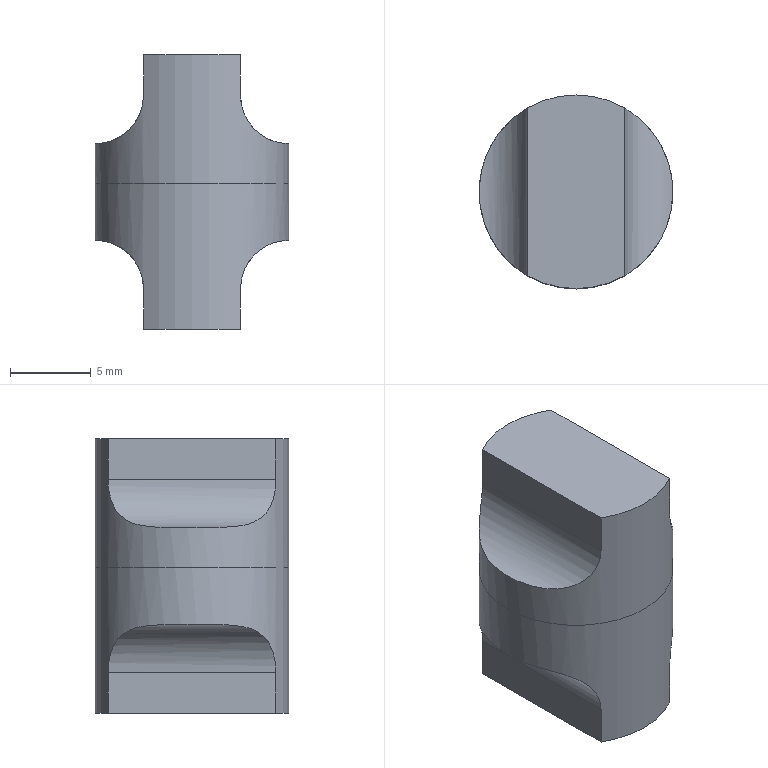Part | NX | 2 solids | 20 faces | box 12 x 12 x 17 mm | volume 1372 mm3 | cylinder 9 | plane 9 | cone 2 | commonest cylinder face diameters 6 x4 5 x2 12 x2 8 x1
STEP:
#1=CARTESIAN_POINT('',(6.,0.,0.));
#2=VERTEX_POINT('',#1);
#3=CARTESIAN_POINT('',(0.,0.,0.));
#4=DIRECTION('',(0.,0.,1.));
#5=DIRECTION('',(1.,0.,0.));
#6=AXIS2_PLACEMENT_3D('',#3,#4,#5);
#7=CIRCLE('',#6,6.);
#8=EDGE_CURVE('',#2,#2,#7,.T.);
#9=ORIENTED_EDGE('',*,*,#8,.T.);
#10=EDGE_LOOP('',(#9));
#11=FACE_BOUND('',#10,.T.);
#12=CARTESIAN_POINT('',(-3.,-5.196,8.));
#13=VERTEX_POINT('',#12);
#14=CARTESIAN_POINT('',(-3.,-5.196,5.5));
#15=VERTEX_POINT('',#14);
#16=CARTESIAN_POINT('',(-3.,-5.196,5.5));
#17=DIRECTION('',(0.,0.,1.));
#18=VECTOR('',#17,1000.);
#19=LINE('',#16,#18);
#20=EDGE_CURVE('',#13,#15,#19,.F.);
#21=ORIENTED_EDGE('',*,*,#20,.T.);
#22=CARTESIAN_POINT('',(-3.,5.196,5.5));
#23=VERTEX_POINT('',#22);
#24=CARTESIAN_POINT('',(-3.,-5.196,5.5));
#25=CARTESIAN_POINT('',(-3.,-5.196,4.839));
#26=CARTESIAN_POINT('',(-3.48,-4.956,3.543));
#27=CARTESIAN_POINT('',(-4.858,-3.707,2.629));
#28=CARTESIAN_POINT('',(-5.786,-1.955,2.492));
#29=CARTESIAN_POINT('',(-6.107,0.008111,2.504));
#30=CARTESIAN_POINT('',(-5.786,1.951,2.491));
#31=CARTESIAN_POINT('',(-4.854,3.713,2.63));
#32=CARTESIAN_POINT('',(-3.479,4.955,3.544));
#33=CARTESIAN_POINT('',(-3.,5.196,4.838));
#34=CARTESIAN_POINT('',(-3.,5.196,5.5));
#35=B_SPLINE_CURVE_WITH_KNOTS('',3,(#24,#25,#26,#27,#28,#29,#30,#31,#32,#33,#34),.UNSPECIFIED.,.F.,.F.,(4,1,1,1,1,1,1,1,4),(-0.007764,-0.005822,-0.00388,-0.001937,0.000004764,0.001947,0.003889,0.005831,0.007773),.UNSPECIFIED.);
#36=EDGE_CURVE('',#15,#23,#35,.T.);
#37=ORIENTED_EDGE('',*,*,#36,.T.);
#38=CARTESIAN_POINT('',(-3.,5.196,8.));
#39=VERTEX_POINT('',#38);
#40=CARTESIAN_POINT('',(-3.,5.196,5.5));
#41=DIRECTION('',(0.,0.,1.));
#42=VECTOR('',#41,1000.);
#43=LINE('',#40,#42);
#44=EDGE_CURVE('',#23,#39,#43,.T.);
#45=ORIENTED_EDGE('',*,*,#44,.T.);
#46=CARTESIAN_POINT('',(3.,5.196,8.));
#47=VERTEX_POINT('',#46);
#48=CARTESIAN_POINT('',(0.,0.,8.));
#49=DIRECTION('',(0.,0.,-1.));
#50=DIRECTION('',(1.,0.,0.));
#51=AXIS2_PLACEMENT_3D('',#48,#49,#50);
#52=CIRCLE('',#51,6.);
#53=EDGE_CURVE('',#39,#47,#52,.T.);
#54=ORIENTED_EDGE('',*,*,#53,.T.);
#55=CARTESIAN_POINT('',(3.,5.196,5.5));
#56=VERTEX_POINT('',#55);
#57=CARTESIAN_POINT('',(3.,5.196,5.5));
#58=DIRECTION('',(0.,0.,1.));
#59=VECTOR('',#58,1000.);
#60=LINE('',#57,#59);
#61=EDGE_CURVE('',#56,#47,#60,.T.);
#62=ORIENTED_EDGE('',*,*,#61,.F.);
#63=CARTESIAN_POINT('',(3.,-5.196,5.5));
#64=VERTEX_POINT('',#63);
#65=CARTESIAN_POINT('',(3.,5.196,5.5));
#66=CARTESIAN_POINT('',(3.,5.196,4.839));
#67=CARTESIAN_POINT('',(3.48,4.956,3.543));
#68=CARTESIAN_POINT('',(4.858,3.707,2.629));
#69=CARTESIAN_POINT('',(5.786,1.955,2.492));
#70=CARTESIAN_POINT('',(6.107,-0.008111,2.504));
#71=CARTESIAN_POINT('',(5.786,-1.951,2.491));
#72=CARTESIAN_POINT('',(4.854,-3.713,2.63));
#73=CARTESIAN_POINT('',(3.479,-4.955,3.544));
#74=CARTESIAN_POINT('',(3.,-5.196,4.838));
#75=CARTESIAN_POINT('',(3.,-5.196,5.5));
#76=B_SPLINE_CURVE_WITH_KNOTS('',3,(#65,#66,#67,#68,#69,#70,#71,#72,#73,#74,#75),.UNSPECIFIED.,.F.,.F.,(4,1,1,1,1,1,1,1,4),(-0.007764,-0.005822,-0.00388,-0.001937,0.000004764,0.001947,0.003889,0.005831,0.007773),.UNSPECIFIED.);
#77=EDGE_CURVE('',#56,#64,#76,.T.);
#78=ORIENTED_EDGE('',*,*,#77,.T.);
#79=CARTESIAN_POINT('',(3.,-5.196,8.));
#80=VERTEX_POINT('',#79);
#81=CARTESIAN_POINT('',(3.,-5.196,5.5));
#82=DIRECTION('',(0.,0.,1.));
#83=VECTOR('',#82,1000.);
#84=LINE('',#81,#83);
#85=EDGE_CURVE('',#80,#64,#84,.F.);
#86=ORIENTED_EDGE('',*,*,#85,.F.);
#87=CARTESIAN_POINT('',(0.,0.,8.));
#88=DIRECTION('',(0.,0.,-1.));
#89=DIRECTION('',(1.,0.,0.));
#90=AXIS2_PLACEMENT_3D('',#87,#88,#89);
#91=CIRCLE('',#90,6.);
#92=EDGE_CURVE('',#80,#13,#91,.T.);
#93=ORIENTED_EDGE('',*,*,#92,.T.);
#94=EDGE_LOOP('',(#21,#37,#45,#54,#62,#78,#86,#93));
#95=FACE_BOUND('',#94,.T.);
#96=CARTESIAN_POINT('',(0.,0.,0.));
#97=DIRECTION('',(0.,0.,1.));
#98=DIRECTION('',(1.,0.,0.));
#99=AXIS2_PLACEMENT_3D('',#96,#97,#98);
#100=CYLINDRICAL_SURFACE('',#99,6.);
#101=ADVANCED_FACE('',(#11,#95),#100,.T.);
#102=CARTESIAN_POINT('',(4.,0.,0.));
#103=VERTEX_POINT('',#102);
#104=CARTESIAN_POINT('',(0.,0.,0.));
#105=DIRECTION('',(0.,0.,-1.));
#106=DIRECTION('',(1.,0.,0.));
#107=AXIS2_PLACEMENT_3D('',#104,#105,#106);
#108=CIRCLE('',#107,4.);
#109=EDGE_CURVE('',#103,#103,#108,.T.);
#110=ORIENTED_EDGE('',*,*,#109,.F.);
#111=EDGE_LOOP('',(#110));
#112=FACE_BOUND('',#111,.T.);
#113=ORIENTED_EDGE('',*,*,#8,.F.);
#114=EDGE_LOOP('',(#113));
#115=FACE_BOUND('',#114,.T.);
#116=CARTESIAN_POINT('',(0.,0.,0.));
#117=DIRECTION('',(0.,0.,-1.));
#118=DIRECTION('',(-1.,0.,0.));
#119=AXIS2_PLACEMENT_3D('',#116,#117,#118);
#120=PLANE('',#119);
#121=ADVANCED_FACE('',(#112,#115),#120,.T.);
#122=CARTESIAN_POINT('',(-2.5,0.,-2.5));
#123=VERTEX_POINT('',#122);
#124=CARTESIAN_POINT('',(0.,0.,-2.5));
#125=DIRECTION('',(0.,0.,-1.));
#126=DIRECTION('',(-1.,0.,0.));
#127=AXIS2_PLACEMENT_3D('',#124,#125,#126);
#128=CIRCLE('',#127,2.5);
#129=EDGE_CURVE('',#123,#123,#128,.F.);
#130=ORIENTED_EDGE('',*,*,#129,.T.);
#131=EDGE_LOOP('',(#130));
#132=FACE_BOUND('',#131,.T.);
#133=CARTESIAN_POINT('',(4.,0.,-2.5));
#134=VERTEX_POINT('',#133);
#135=CARTESIAN_POINT('',(0.,0.,-2.5));
#136=DIRECTION('',(0.,0.,1.));
#137=DIRECTION('',(1.,0.,0.));
#138=AXIS2_PLACEMENT_3D('',#135,#136,#137);
#139=CIRCLE('',#138,4.);
#140=EDGE_CURVE('',#134,#134,#139,.T.);
#141=ORIENTED_EDGE('',*,*,#140,.F.);
#142=EDGE_LOOP('',(#141));
#143=FACE_BOUND('',#142,.T.);
#144=CARTESIAN_POINT('',(0.,0.,-2.5));
#145=DIRECTION('',(0.,0.,-1.));
#146=DIRECTION('',(-1.,0.,0.));
#147=AXIS2_PLACEMENT_3D('',#144,#145,#146);
#148=PLANE('',#147);
#149=ADVANCED_FACE('',(#132,#143),#148,.T.);
#150=ORIENTED_EDGE('',*,*,#140,.T.);
#151=EDGE_LOOP('',(#150));
#152=FACE_BOUND('',#151,.T.);
#153=ORIENTED_EDGE('',*,*,#109,.T.);
#154=EDGE_LOOP('',(#153));
#155=FACE_BOUND('',#154,.T.);
#156=CARTESIAN_POINT('',(0.,0.,0.));
#157=DIRECTION('',(0.,0.,-1.));
#158=DIRECTION('',(1.,0.,0.));
#159=AXIS2_PLACEMENT_3D('',#156,#157,#158);
#160=CYLINDRICAL_SURFACE('',#159,4.);
#161=ADVANCED_FACE('',(#152,#155),#160,.T.);
#162=ORIENTED_EDGE('',*,*,#44,.F.);
#163=CARTESIAN_POINT('',(-3.,-5.196,5.5));
#164=DIRECTION('',(0.,1.,0.));
#165=VECTOR('',#164,1000.);
#166=LINE('',#163,#165);
#167=EDGE_CURVE('',#23,#15,#166,.F.);
#168=ORIENTED_EDGE('',*,*,#167,.T.);
#169=ORIENTED_EDGE('',*,*,#20,.F.);
#170=CARTESIAN_POINT('',(-3.,-5.196,8.));
#171=DIRECTION('',(0.,1.,0.));
#172=VECTOR('',#171,1000.);
#173=LINE('',#170,#172);
#174=EDGE_CURVE('',#13,#39,#173,.T.);
#175=ORIENTED_EDGE('',*,*,#174,.T.);
#176=EDGE_LOOP('',(#162,#168,#169,#175));
#177=FACE_BOUND('',#176,.T.);
#178=CARTESIAN_POINT('',(-3.,-5.196,5.5));
#179=DIRECTION('',(1.,0.,0.));
#180=DIRECTION('',(0.,0.,-1.));
#181=AXIS2_PLACEMENT_3D('',#178,#179,#180);
#182=PLANE('',#181);
#183=ADVANCED_FACE('',(#177),#182,.F.);
#184=ORIENTED_EDGE('',*,*,#85,.T.);
#185=CARTESIAN_POINT('',(3.,5.196,5.5));
#186=DIRECTION('',(0.,-1.,0.));
#187=VECTOR('',#186,1000.);
#188=LINE('',#185,#187);
#189=EDGE_CURVE('',#64,#56,#188,.F.);
#190=ORIENTED_EDGE('',*,*,#189,.T.);
#191=ORIENTED_EDGE('',*,*,#61,.T.);
#192=CARTESIAN_POINT('',(3.,5.196,8.));
#193=DIRECTION('',(0.,-1.,0.));
#194=VECTOR('',#193,1000.);
#195=LINE('',#192,#194);
#196=EDGE_CURVE('',#47,#80,#195,.T.);
#197=ORIENTED_EDGE('',*,*,#196,.T.);
#198=EDGE_LOOP('',(#184,#190,#191,#197));
#199=FACE_BOUND('',#198,.T.);
#200=CARTESIAN_POINT('',(3.,5.196,5.5));
#201=DIRECTION('',(-1.,0.,0.));
#202=DIRECTION('',(0.,0.,1.));
#203=AXIS2_PLACEMENT_3D('',#200,#201,#202);
#204=PLANE('',#203);
#205=ADVANCED_FACE('',(#199),#204,.F.);
#206=ORIENTED_EDGE('',*,*,#174,.F.);
#207=ORIENTED_EDGE('',*,*,#92,.F.);
#208=ORIENTED_EDGE('',*,*,#196,.F.);
#209=ORIENTED_EDGE('',*,*,#53,.F.);
#210=EDGE_LOOP('',(#206,#207,#208,#209));
#211=FACE_BOUND('',#210,.T.);
#212=CARTESIAN_POINT('',(0.,0.,8.));
#213=DIRECTION('',(0.,0.,-1.));
#214=DIRECTION('',(-1.,0.,0.));
#215=AXIS2_PLACEMENT_3D('',#212,#213,#214);
#216=PLANE('',#215);
#217=ADVANCED_FACE('',(#211),#216,.F.);
#218=ORIENTED_EDGE('',*,*,#36,.F.);
#219=ORIENTED_EDGE('',*,*,#167,.F.);
#220=EDGE_LOOP('',(#218,#219));
#221=FACE_BOUND('',#220,.T.);
#222=CARTESIAN_POINT('',(-6.,0.,5.5));
#223=DIRECTION('',(0.,1.,0.));
#224=DIRECTION('',(0.,0.,1.));
#225=AXIS2_PLACEMENT_3D('',#222,#223,#224);
#226=CYLINDRICAL_SURFACE('',#225,3.);
#227=ADVANCED_FACE('',(#221),#226,.F.);
#228=ORIENTED_EDGE('',*,*,#77,.F.);
#229=ORIENTED_EDGE('',*,*,#189,.F.);
#230=EDGE_LOOP('',(#228,#229));
#231=FACE_BOUND('',#230,.T.);
#232=CARTESIAN_POINT('',(6.,0.,5.5));
#233=DIRECTION('',(0.,-1.,0.));
#234=DIRECTION('',(0.,0.,-1.));
#235=AXIS2_PLACEMENT_3D('',#232,#233,#234);
#236=CYLINDRICAL_SURFACE('',#235,3.);
#237=ADVANCED_FACE('',(#231),#236,.F.);
#238=CARTESIAN_POINT('',(-2.5,0.,3.8));
#239=VERTEX_POINT('',#238);
#240=CARTESIAN_POINT('',(0.,0.,3.8));
#241=DIRECTION('',(0.,0.,-1.));
#242=DIRECTION('',(-1.,0.,0.));
#243=AXIS2_PLACEMENT_3D('',#240,#241,#242);
#244=CIRCLE('',#243,2.5);
#245=EDGE_CURVE('',#239,#239,#244,.T.);
#246=ORIENTED_EDGE('',*,*,#245,.T.);
#247=EDGE_LOOP('',(#246));
#248=FACE_BOUND('',#247,.T.);
#249=CARTESIAN_POINT('',(0.,0.,5.303));
#250=VERTEX_POINT('',#249);
#251=VERTEX_LOOP('',#250);
#252=FACE_BOUND('',#251,.T.);
#253=CARTESIAN_POINT('',(0.,0.,3.5));
#254=DIRECTION('',(0.,0.,-1.));
#255=DIRECTION('',(-1.,0.,0.));
#256=AXIS2_PLACEMENT_3D('',#253,#254,#255);
#257=CONICAL_SURFACE('',#256,3.,1.03);
#258=ADVANCED_FACE('',(#248,#252),#257,.F.);
#259=ORIENTED_EDGE('',*,*,#245,.F.);
#260=EDGE_LOOP('',(#259));
#261=FACE_BOUND('',#260,.T.);
#262=ORIENTED_EDGE('',*,*,#129,.F.);
#263=EDGE_LOOP('',(#262));
#264=FACE_BOUND('',#263,.T.);
#265=CARTESIAN_POINT('',(0.,0.,-2.5));
#266=DIRECTION('',(0.,0.,1.));
#267=DIRECTION('',(1.,0.,0.));
#268=AXIS2_PLACEMENT_3D('',#265,#266,#267);
#269=CYLINDRICAL_SURFACE('',#268,2.5);
#270=ADVANCED_FACE('',(#261,#264),#269,.F.);
#271=CLOSED_SHELL('',(#101,#121,#149,#161,#183,#205,#217,#227,#237,#258,#270));
#272=MANIFOLD_SOLID_BREP('',#271);
#273=CARTESIAN_POINT('',(3.,5.196,-6.5));
#274=VERTEX_POINT('',#273);
#275=CARTESIAN_POINT('',(3.,5.196,-9.));
#276=VERTEX_POINT('',#275);
#277=CARTESIAN_POINT('',(3.,5.196,-9.));
#278=DIRECTION('',(0.,0.,1.));
#279=VECTOR('',#278,1000.);
#280=LINE('',#277,#279);
#281=EDGE_CURVE('',#274,#276,#280,.F.);
#282=ORIENTED_EDGE('',*,*,#281,.F.);
#283=CARTESIAN_POINT('',(3.,-5.196,-6.5));
#284=VERTEX_POINT('',#283);
#285=CARTESIAN_POINT('',(3.,5.196,-6.5));
#286=DIRECTION('',(0.,-1.,0.));
#287=VECTOR('',#286,1000.);
#288=LINE('',#285,#287);
#289=EDGE_CURVE('',#274,#284,#288,.T.);
#290=ORIENTED_EDGE('',*,*,#289,.T.);
#291=CARTESIAN_POINT('',(3.,-5.196,-9.));
#292=VERTEX_POINT('',#291);
#293=CARTESIAN_POINT('',(3.,-5.196,-9.));
#294=DIRECTION('',(0.,0.,1.));
#295=VECTOR('',#294,1000.);
#296=LINE('',#293,#295);
#297=EDGE_CURVE('',#292,#284,#296,.T.);
#298=ORIENTED_EDGE('',*,*,#297,.F.);
#299=CARTESIAN_POINT('',(3.,5.196,-9.));
#300=DIRECTION('',(0.,-1.,0.));
#301=VECTOR('',#300,1000.);
#302=LINE('',#299,#301);
#303=EDGE_CURVE('',#276,#292,#302,.T.);
#304=ORIENTED_EDGE('',*,*,#303,.F.);
#305=EDGE_LOOP('',(#282,#290,#298,#304));
#306=FACE_BOUND('',#305,.T.);
#307=CARTESIAN_POINT('',(3.,5.196,-9.));
#308=DIRECTION('',(-1.,0.,0.));
#309=DIRECTION('',(0.,0.,1.));
#310=AXIS2_PLACEMENT_3D('',#307,#308,#309);
#311=PLANE('',#310);
#312=ADVANCED_FACE('',(#306),#311,.F.);
#313=CARTESIAN_POINT('',(-3.,-5.196,-6.5));
#314=VERTEX_POINT('',#313);
#315=CARTESIAN_POINT('',(-3.,-5.196,-9.));
#316=VERTEX_POINT('',#315);
#317=CARTESIAN_POINT('',(-3.,-5.196,-9.));
#318=DIRECTION('',(0.,0.,1.));
#319=VECTOR('',#318,1000.);
#320=LINE('',#317,#319);
#321=EDGE_CURVE('',#314,#316,#320,.F.);
#322=ORIENTED_EDGE('',*,*,#321,.F.);
#323=CARTESIAN_POINT('',(-3.,5.196,-6.5));
#324=VERTEX_POINT('',#323);
#325=CARTESIAN_POINT('',(-3.,-5.196,-6.5));
#326=DIRECTION('',(0.,1.,0.));
#327=VECTOR('',#326,1000.);
#328=LINE('',#325,#327);
#329=EDGE_CURVE('',#314,#324,#328,.T.);
#330=ORIENTED_EDGE('',*,*,#329,.T.);
#331=CARTESIAN_POINT('',(-3.,5.196,-9.));
#332=VERTEX_POINT('',#331);
#333=CARTESIAN_POINT('',(-3.,5.196,-9.));
#334=DIRECTION('',(0.,0.,1.));
#335=VECTOR('',#334,1000.);
#336=LINE('',#333,#335);
#337=EDGE_CURVE('',#332,#324,#336,.T.);
#338=ORIENTED_EDGE('',*,*,#337,.F.);
#339=CARTESIAN_POINT('',(-3.,-5.196,-9.));
#340=DIRECTION('',(0.,1.,0.));
#341=VECTOR('',#340,1000.);
#342=LINE('',#339,#341);
#343=EDGE_CURVE('',#316,#332,#342,.T.);
#344=ORIENTED_EDGE('',*,*,#343,.F.);
#345=EDGE_LOOP('',(#322,#330,#338,#344));
#346=FACE_BOUND('',#345,.T.);
#347=CARTESIAN_POINT('',(-3.,-5.196,-9.));
#348=DIRECTION('',(1.,0.,0.));
#349=DIRECTION('',(0.,0.,-1.));
#350=AXIS2_PLACEMENT_3D('',#347,#348,#349);
#351=PLANE('',#350);
#352=ADVANCED_FACE('',(#346),#351,.F.);
#353=ORIENTED_EDGE('',*,*,#337,.T.);
#354=CARTESIAN_POINT('',(-3.,5.196,-6.5));
#355=CARTESIAN_POINT('',(-3.,5.196,-5.839));
#356=CARTESIAN_POINT('',(-3.48,4.956,-4.543));
#357=CARTESIAN_POINT('',(-4.858,3.707,-3.629));
#358=CARTESIAN_POINT('',(-5.786,1.955,-3.492));
#359=CARTESIAN_POINT('',(-6.107,-0.008111,-3.504));
#360=CARTESIAN_POINT('',(-5.786,-1.951,-3.491));
#361=CARTESIAN_POINT('',(-4.854,-3.713,-3.63));
#362=CARTESIAN_POINT('',(-3.479,-4.955,-4.544));
#363=CARTESIAN_POINT('',(-3.,-5.196,-5.838));
#364=CARTESIAN_POINT('',(-3.,-5.196,-6.5));
#365=B_SPLINE_CURVE_WITH_KNOTS('',3,(#354,#355,#356,#357,#358,#359,#360,#361,#362,#363,#364),.UNSPECIFIED.,.F.,.F.,(4,1,1,1,1,1,1,1,4),(0.,0.001956,0.003911,0.005867,0.007822,0.009778,0.01173,0.01369,0.01564),.UNSPECIFIED.);
#366=EDGE_CURVE('',#324,#314,#365,.T.);
#367=ORIENTED_EDGE('',*,*,#366,.T.);
#368=ORIENTED_EDGE('',*,*,#321,.T.);
#369=CARTESIAN_POINT('',(0.,0.,-9.));
#370=DIRECTION('',(0.,0.,-1.));
#371=DIRECTION('',(1.,0.,0.));
#372=AXIS2_PLACEMENT_3D('',#369,#370,#371);
#373=CIRCLE('',#372,6.);
#374=EDGE_CURVE('',#292,#316,#373,.T.);
#375=ORIENTED_EDGE('',*,*,#374,.F.);
#376=ORIENTED_EDGE('',*,*,#297,.T.);
#377=CARTESIAN_POINT('',(3.,-5.196,-6.5));
#378=CARTESIAN_POINT('',(3.,-5.196,-5.839));
#379=CARTESIAN_POINT('',(3.48,-4.956,-4.543));
#380=CARTESIAN_POINT('',(4.858,-3.707,-3.629));
#381=CARTESIAN_POINT('',(5.786,-1.955,-3.492));
#382=CARTESIAN_POINT('',(6.107,0.008111,-3.504));
#383=CARTESIAN_POINT('',(5.786,1.951,-3.491));
#384=CARTESIAN_POINT('',(4.854,3.713,-3.63));
#385=CARTESIAN_POINT('',(3.479,4.955,-4.544));
#386=CARTESIAN_POINT('',(3.,5.196,-5.838));
#387=CARTESIAN_POINT('',(3.,5.196,-6.5));
#388=B_SPLINE_CURVE_WITH_KNOTS('',3,(#377,#378,#379,#380,#381,#382,#383,#384,#385,#386,#387),.UNSPECIFIED.,.F.,.F.,(4,1,1,1,1,1,1,1,4),(0.,0.001956,0.003911,0.005867,0.007822,0.009778,0.01173,0.01369,0.01564),.UNSPECIFIED.);
#389=EDGE_CURVE('',#284,#274,#388,.T.);
#390=ORIENTED_EDGE('',*,*,#389,.T.);
#391=ORIENTED_EDGE('',*,*,#281,.T.);
#392=CARTESIAN_POINT('',(0.,0.,-9.));
#393=DIRECTION('',(0.,0.,-1.));
#394=DIRECTION('',(1.,0.,0.));
#395=AXIS2_PLACEMENT_3D('',#392,#393,#394);
#396=CIRCLE('',#395,6.);
#397=EDGE_CURVE('',#332,#276,#396,.T.);
#398=ORIENTED_EDGE('',*,*,#397,.F.);
#399=EDGE_LOOP('',(#353,#367,#368,#375,#376,#390,#391,#398));
#400=FACE_BOUND('',#399,.T.);
#401=CARTESIAN_POINT('',(6.,0.,0.));
#402=VERTEX_POINT('',#401);
#403=CARTESIAN_POINT('',(0.,0.,0.));
#404=DIRECTION('',(0.,0.,-1.));
#405=DIRECTION('',(1.,0.,0.));
#406=AXIS2_PLACEMENT_3D('',#403,#404,#405);
#407=CIRCLE('',#406,6.);
#408=EDGE_CURVE('',#402,#402,#407,.T.);
#409=ORIENTED_EDGE('',*,*,#408,.T.);
#410=EDGE_LOOP('',(#409));
#411=FACE_BOUND('',#410,.T.);
#412=CARTESIAN_POINT('',(0.,0.,-9.));
#413=DIRECTION('',(0.,0.,1.));
#414=DIRECTION('',(1.,0.,0.));
#415=AXIS2_PLACEMENT_3D('',#412,#413,#414);
#416=CYLINDRICAL_SURFACE('',#415,6.);
#417=ADVANCED_FACE('',(#400,#411),#416,.T.);
#418=ORIENTED_EDGE('',*,*,#303,.T.);
#419=ORIENTED_EDGE('',*,*,#374,.T.);
#420=ORIENTED_EDGE('',*,*,#343,.T.);
#421=ORIENTED_EDGE('',*,*,#397,.T.);
#422=EDGE_LOOP('',(#418,#419,#420,#421));
#423=FACE_BOUND('',#422,.T.);
#424=CARTESIAN_POINT('',(0.,0.,-9.));
#425=DIRECTION('',(0.,0.,-1.));
#426=DIRECTION('',(-1.,0.,0.));
#427=AXIS2_PLACEMENT_3D('',#424,#425,#426);
#428=PLANE('',#427);
#429=ADVANCED_FACE('',(#423),#428,.T.);
#430=CARTESIAN_POINT('',(2.5,0.,0.));
#431=VERTEX_POINT('',#430);
#432=CARTESIAN_POINT('',(0.,0.,0.));
#433=DIRECTION('',(0.,0.,1.));
#434=DIRECTION('',(1.,0.,0.));
#435=AXIS2_PLACEMENT_3D('',#432,#433,#434);
#436=CIRCLE('',#435,2.5);
#437=EDGE_CURVE('',#431,#431,#436,.F.);
#438=ORIENTED_EDGE('',*,*,#437,.T.);
#439=EDGE_LOOP('',(#438));
#440=FACE_BOUND('',#439,.T.);
#441=ORIENTED_EDGE('',*,*,#408,.F.);
#442=EDGE_LOOP('',(#441));
#443=FACE_BOUND('',#442,.T.);
#444=CARTESIAN_POINT('',(0.,0.,0.));
#445=DIRECTION('',(0.,0.,1.));
#446=DIRECTION('',(1.,0.,0.));
#447=AXIS2_PLACEMENT_3D('',#444,#445,#446);
#448=PLANE('',#447);
#449=ADVANCED_FACE('',(#440,#443),#448,.T.);
#450=ORIENTED_EDGE('',*,*,#289,.F.);
#451=ORIENTED_EDGE('',*,*,#389,.F.);
#452=EDGE_LOOP('',(#450,#451));
#453=FACE_BOUND('',#452,.T.);
#454=CARTESIAN_POINT('',(6.,5.196,-6.5));
#455=DIRECTION('',(0.,-1.,0.));
#456=DIRECTION('',(0.,0.,-1.));
#457=AXIS2_PLACEMENT_3D('',#454,#455,#456);
#458=CYLINDRICAL_SURFACE('',#457,3.);
#459=ADVANCED_FACE('',(#453),#458,.F.);
#460=ORIENTED_EDGE('',*,*,#329,.F.);
#461=ORIENTED_EDGE('',*,*,#366,.F.);
#462=EDGE_LOOP('',(#460,#461));
#463=FACE_BOUND('',#462,.T.);
#464=CARTESIAN_POINT('',(-6.,-5.196,-6.5));
#465=DIRECTION('',(0.,1.,0.));
#466=DIRECTION('',(0.,0.,1.));
#467=AXIS2_PLACEMENT_3D('',#464,#465,#466);
#468=CYLINDRICAL_SURFACE('',#467,3.);
#469=ADVANCED_FACE('',(#463),#468,.F.);
#470=CARTESIAN_POINT('',(2.5,0.,-6.03));
#471=VERTEX_POINT('',#470);
#472=CARTESIAN_POINT('',(0.,0.,-6.03));
#473=DIRECTION('',(0.,0.,1.));
#474=DIRECTION('',(1.,0.,0.));
#475=AXIS2_PLACEMENT_3D('',#472,#473,#474);
#476=CIRCLE('',#475,2.5);
#477=EDGE_CURVE('',#471,#471,#476,.T.);
#478=ORIENTED_EDGE('',*,*,#477,.T.);
#479=EDGE_LOOP('',(#478));
#480=FACE_BOUND('',#479,.T.);
#481=CARTESIAN_POINT('',(0.,0.,-7.532));
#482=VERTEX_POINT('',#481);
#483=VERTEX_LOOP('',#482);
#484=FACE_BOUND('',#483,.T.);
#485=CARTESIAN_POINT('',(0.,0.,-6.));
#486=DIRECTION('',(0.,0.,1.));
#487=DIRECTION('',(1.,0.,0.));
#488=AXIS2_PLACEMENT_3D('',#485,#486,#487);
#489=CONICAL_SURFACE('',#488,2.55,1.03);
#490=ADVANCED_FACE('',(#480,#484),#489,.F.);
#491=ORIENTED_EDGE('',*,*,#477,.F.);
#492=EDGE_LOOP('',(#491));
#493=FACE_BOUND('',#492,.T.);
#494=ORIENTED_EDGE('',*,*,#437,.F.);
#495=EDGE_LOOP('',(#494));
#496=FACE_BOUND('',#495,.T.);
#497=CARTESIAN_POINT('',(0.,0.,0.));
#498=DIRECTION('',(0.,0.,-1.));
#499=DIRECTION('',(-1.,0.,0.));
#500=AXIS2_PLACEMENT_3D('',#497,#498,#499);
#501=CYLINDRICAL_SURFACE('',#500,2.5);
#502=ADVANCED_FACE('',(#493,#496),#501,.F.);
#503=CLOSED_SHELL('',(#312,#352,#417,#429,#449,#459,#469,#490,#502));
#504=MANIFOLD_SOLID_BREP('',#503);
#505=(LENGTH_UNIT()NAMED_UNIT(*)SI_UNIT(.MILLI.,.METRE.));
#506=UNCERTAINTY_MEASURE_WITH_UNIT(LENGTH_MEASURE(0.0508),#505,'','');
#507=(NAMED_UNIT(*)PLANE_ANGLE_UNIT()SI_UNIT($,.RADIAN.));
#508=(NAMED_UNIT(*)SI_UNIT($,.STERADIAN.)SOLID_ANGLE_UNIT());
#509=(GEOMETRIC_REPRESENTATION_CONTEXT(3)GLOBAL_UNCERTAINTY_ASSIGNED_CONTEXT((#506))GLOBAL_UNIT_ASSIGNED_CONTEXT((#505,#507,#508))REPRESENTATION_CONTEXT('',''));
#510=ADVANCED_BREP_SHAPE_REPRESENTATION('',(#272,#504),#509);